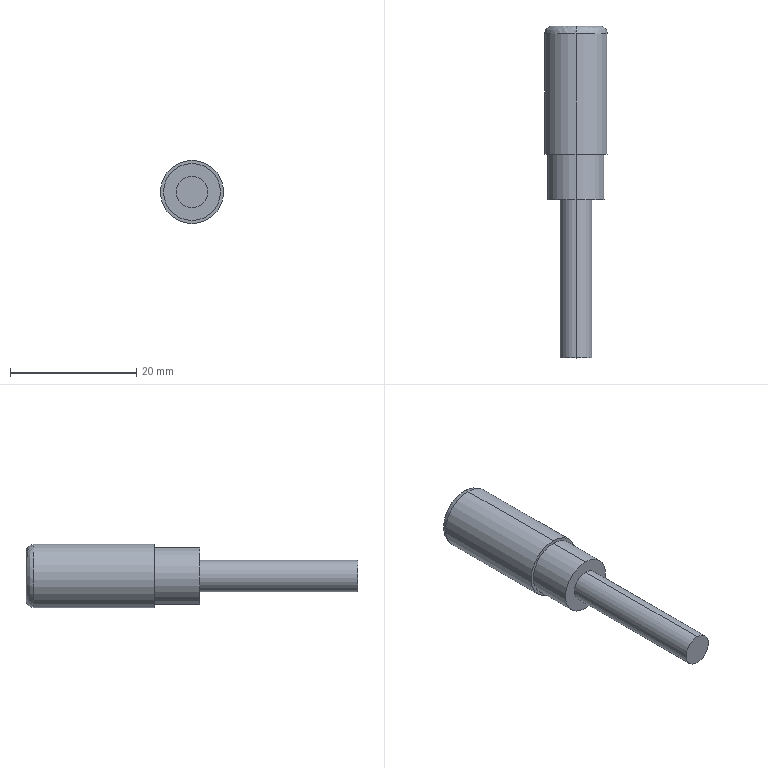Part | SolidWorks | features ICE 3, BaseBody 1 | 1 solid | 19 faces | box 10 x 52.5 x 10 mm | volume 2526 mm3 | plane 11 | cylinder 6 | spline 2 | commonest cylinder face diameters 5 x2 9 x2 10 x2
STEP:
#1=CARTESIAN_POINT('',(0.,24.5,3.8));
#2=VERTEX_POINT('',#1);
#3=CARTESIAN_POINT('',(0.,24.5,-3.8));
#4=VERTEX_POINT('',#3);
#5=CARTESIAN_POINT('',(0.,24.5,3.8));
#6=CARTESIAN_POINT('',(-7.6,24.5,3.8));
#7=CARTESIAN_POINT('',(-7.6,24.5,-3.8));
#8=CARTESIAN_POINT('',(0.,24.5,-3.8));
#9=(BOUNDED_CURVE()B_SPLINE_CURVE(3,(#5,#6,#7,#8),.UNSPECIFIED.,.F.,.F.)B_SPLINE_CURVE_WITH_KNOTS((4,4),(0.,1.),.UNSPECIFIED.)CURVE()GEOMETRIC_REPRESENTATION_ITEM()RATIONAL_B_SPLINE_CURVE((1.,0.3333,0.3333,1.))REPRESENTATION_ITEM(''));
#10=EDGE_CURVE('',#2,#4,#9,.T.);
#11=ORIENTED_EDGE('',*,*,#10,.T.);
#12=CARTESIAN_POINT('',(0.,23.3,-5.));
#13=VERTEX_POINT('',#12);
#14=CARTESIAN_POINT('',(0.,23.3,-3.8));
#15=DIRECTION('',(-1.,0.,0.));
#16=DIRECTION('',(0.,0.,-1.));
#17=AXIS2_PLACEMENT_3D('',#14,#15,#16);
#18=CIRCLE('',#17,1.2);
#19=EDGE_CURVE('',#4,#13,#18,.T.);
#20=ORIENTED_EDGE('',*,*,#19,.T.);
#21=CARTESIAN_POINT('',(0.,23.3,5.));
#22=VERTEX_POINT('',#21);
#23=CARTESIAN_POINT('',(0.,23.3,0.));
#24=DIRECTION('',(0.,-1.,0.));
#25=DIRECTION('',(0.,0.,-1.));
#26=AXIS2_PLACEMENT_3D('',#23,#24,#25);
#27=CIRCLE('',#26,5.);
#28=EDGE_CURVE('',#22,#13,#27,.T.);
#29=ORIENTED_EDGE('',*,*,#28,.F.);
#30=CARTESIAN_POINT('',(0.,23.3,3.8));
#31=DIRECTION('',(1.,0.,0.));
#32=DIRECTION('',(0.,0.,1.));
#33=AXIS2_PLACEMENT_3D('',#30,#31,#32);
#34=CIRCLE('',#33,1.2);
#35=EDGE_CURVE('',#2,#22,#34,.T.);
#36=ORIENTED_EDGE('',*,*,#35,.F.);
#37=EDGE_LOOP('',(#11,#20,#29,#36));
#38=FACE_OUTER_BOUND('',#37,.T.);
#39=CARTESIAN_POINT('',(0.,24.5,-3.8));
#40=CARTESIAN_POINT('',(-7.6,24.5,-3.8));
#41=CARTESIAN_POINT('',(-7.6,24.5,3.8));
#42=CARTESIAN_POINT('',(0.,24.5,3.8));
#43=CARTESIAN_POINT('',(0.,24.5,-4.503));
#44=CARTESIAN_POINT('',(-9.006,24.5,-4.503));
#45=CARTESIAN_POINT('',(-9.006,24.5,4.503));
#46=CARTESIAN_POINT('',(0.,24.5,4.503));
#47=CARTESIAN_POINT('',(0.,24.003,-5.));
#48=CARTESIAN_POINT('',(-10.,24.003,-5.));
#49=CARTESIAN_POINT('',(-10.,24.003,5.));
#50=CARTESIAN_POINT('',(0.,24.003,5.));
#51=CARTESIAN_POINT('',(0.,23.3,-5.));
#52=CARTESIAN_POINT('',(-10.,23.3,-5.));
#53=CARTESIAN_POINT('',(-10.,23.3,5.));
#54=CARTESIAN_POINT('',(0.,23.3,5.));
#55=(BOUNDED_SURFACE()B_SPLINE_SURFACE(3,3,((#39,#40,#41,#42),(#43,#44,#45,#46),(#47,#48,#49,#50),(#51,#52,#53,#54)),.UNSPECIFIED.,.F.,.F.,.F.)B_SPLINE_SURFACE_WITH_KNOTS((4,4),(4,4),(0.,1.),(0.,1.),.UNSPECIFIED.)GEOMETRIC_REPRESENTATION_ITEM()RATIONAL_B_SPLINE_SURFACE(((1.,0.3333,0.3333,1.),(0.8047,0.2682,0.2682,0.8047),(0.8047,0.2682,0.2682,0.8047),(1.,0.3333,0.3333,1.)))REPRESENTATION_ITEM('')SURFACE());
#56=ADVANCED_FACE('',(#38),#55,.T.);
#57=CARTESIAN_POINT('',(0.,-3.,2.5));
#58=VERTEX_POINT('',#57);
#59=CARTESIAN_POINT('',(0.,-3.,-2.5));
#60=VERTEX_POINT('',#59);
#61=CARTESIAN_POINT('',(0.,-3.,0.));
#62=DIRECTION('',(0.,1.,0.));
#63=DIRECTION('',(0.,0.,-1.));
#64=AXIS2_PLACEMENT_3D('',#61,#62,#63);
#65=CIRCLE('',#64,2.5);
#66=EDGE_CURVE('',#58,#60,#65,.T.);
#67=ORIENTED_EDGE('',*,*,#66,.F.);
#68=CARTESIAN_POINT('',(0.,-28.,2.5));
#69=VERTEX_POINT('',#68);
#70=CARTESIAN_POINT('',(0.,-12.284,2.5));
#71=DIRECTION('',(0.,-1.,0.));
#72=VECTOR('',#71,1000.);
#73=LINE('',#70,#72);
#74=EDGE_CURVE('',#58,#69,#73,.T.);
#75=ORIENTED_EDGE('',*,*,#74,.T.);
#76=CARTESIAN_POINT('',(0.,-28.,-2.5));
#77=VERTEX_POINT('',#76);
#78=CARTESIAN_POINT('',(0.,-28.,0.));
#79=DIRECTION('',(0.,-1.,0.));
#80=DIRECTION('',(0.,0.,-1.));
#81=AXIS2_PLACEMENT_3D('',#78,#79,#80);
#82=CIRCLE('',#81,2.5);
#83=EDGE_CURVE('',#77,#69,#82,.T.);
#84=ORIENTED_EDGE('',*,*,#83,.F.);
#85=CARTESIAN_POINT('',(0.,-12.284,-2.5));
#86=DIRECTION('',(0.,-1.,0.));
#87=VECTOR('',#86,1000.);
#88=LINE('',#85,#87);
#89=EDGE_CURVE('',#60,#77,#88,.T.);
#90=ORIENTED_EDGE('',*,*,#89,.F.);
#91=EDGE_LOOP('',(#67,#75,#84,#90));
#92=FACE_OUTER_BOUND('',#91,.T.);
#93=CARTESIAN_POINT('',(0.,-12.284,0.));
#94=DIRECTION('',(0.,-1.,0.));
#95=DIRECTION('',(0.,0.,-1.));
#96=AXIS2_PLACEMENT_3D('',#93,#94,#95);
#97=CYLINDRICAL_SURFACE('',#96,2.5);
#98=ADVANCED_FACE('',(#92),#97,.T.);
#99=CARTESIAN_POINT('',(0.,4.2,-4.5));
#100=VERTEX_POINT('',#99);
#101=CARTESIAN_POINT('',(0.,4.2,4.5));
#102=VERTEX_POINT('',#101);
#103=CARTESIAN_POINT('',(0.,4.2,0.));
#104=DIRECTION('',(0.,-1.,0.));
#105=DIRECTION('',(0.,0.,-1.));
#106=AXIS2_PLACEMENT_3D('',#103,#104,#105);
#107=CIRCLE('',#106,4.5);
#108=EDGE_CURVE('',#100,#102,#107,.T.);
#109=ORIENTED_EDGE('',*,*,#108,.T.);
#110=CARTESIAN_POINT('',(0.,-3.,4.5));
#111=VERTEX_POINT('',#110);
#112=CARTESIAN_POINT('',(0.,4.2,4.5));
#113=DIRECTION('',(0.,-1.,0.));
#114=VECTOR('',#113,1000.);
#115=LINE('',#112,#114);
#116=EDGE_CURVE('',#102,#111,#115,.T.);
#117=ORIENTED_EDGE('',*,*,#116,.T.);
#118=CARTESIAN_POINT('',(0.,-3.,-4.5));
#119=VERTEX_POINT('',#118);
#120=CARTESIAN_POINT('',(0.,-3.,0.));
#121=DIRECTION('',(0.,-1.,0.));
#122=DIRECTION('',(0.,0.,-1.));
#123=AXIS2_PLACEMENT_3D('',#120,#121,#122);
#124=CIRCLE('',#123,4.5);
#125=EDGE_CURVE('',#119,#111,#124,.T.);
#126=ORIENTED_EDGE('',*,*,#125,.F.);
#127=CARTESIAN_POINT('',(0.,4.2,-4.5));
#128=DIRECTION('',(0.,-1.,0.));
#129=VECTOR('',#128,1000.);
#130=LINE('',#127,#129);
#131=EDGE_CURVE('',#100,#119,#130,.T.);
#132=ORIENTED_EDGE('',*,*,#131,.F.);
#133=EDGE_LOOP('',(#109,#117,#126,#132));
#134=FACE_OUTER_BOUND('',#133,.T.);
#135=CARTESIAN_POINT('',(0.,4.2,0.));
#136=DIRECTION('',(0.,-1.,0.));
#137=DIRECTION('',(0.,0.,-1.));
#138=AXIS2_PLACEMENT_3D('',#135,#136,#137);
#139=CYLINDRICAL_SURFACE('',#138,4.5);
#140=ADVANCED_FACE('',(#134),#139,.T.);
#141=CARTESIAN_POINT('',(0.,23.3,0.));
#142=DIRECTION('',(0.,-1.,0.));
#143=DIRECTION('',(0.,0.,-1.));
#144=AXIS2_PLACEMENT_3D('',#141,#142,#143);
#145=CIRCLE('',#144,5.);
#146=EDGE_CURVE('',#13,#22,#145,.T.);
#147=ORIENTED_EDGE('',*,*,#146,.T.);
#148=CARTESIAN_POINT('',(0.,4.2,5.));
#149=VERTEX_POINT('',#148);
#150=CARTESIAN_POINT('',(0.,11.827,5.));
#151=DIRECTION('',(0.,-1.,0.));
#152=VECTOR('',#151,1000.);
#153=LINE('',#150,#152);
#154=EDGE_CURVE('',#22,#149,#153,.T.);
#155=ORIENTED_EDGE('',*,*,#154,.T.);
#156=CARTESIAN_POINT('',(0.,4.2,-5.));
#157=VERTEX_POINT('',#156);
#158=CARTESIAN_POINT('',(0.,4.2,0.));
#159=DIRECTION('',(0.,-1.,0.));
#160=DIRECTION('',(0.,0.,-1.));
#161=AXIS2_PLACEMENT_3D('',#158,#159,#160);
#162=CIRCLE('',#161,5.);
#163=EDGE_CURVE('',#157,#149,#162,.T.);
#164=ORIENTED_EDGE('',*,*,#163,.F.);
#165=CARTESIAN_POINT('',(0.,11.827,-5.));
#166=DIRECTION('',(0.,-1.,0.));
#167=VECTOR('',#166,1000.);
#168=LINE('',#165,#167);
#169=EDGE_CURVE('',#13,#157,#168,.T.);
#170=ORIENTED_EDGE('',*,*,#169,.F.);
#171=EDGE_LOOP('',(#147,#155,#164,#170));
#172=FACE_OUTER_BOUND('',#171,.T.);
#173=CARTESIAN_POINT('',(0.,11.827,0.));
#174=DIRECTION('',(0.,-1.,0.));
#175=DIRECTION('',(0.,0.,-1.));
#176=AXIS2_PLACEMENT_3D('',#173,#174,#175);
#177=CYLINDRICAL_SURFACE('',#176,5.);
#178=ADVANCED_FACE('',(#172),#177,.T.);
#179=ORIENTED_EDGE('',*,*,#154,.F.);
#180=ORIENTED_EDGE('',*,*,#28,.T.);
#181=ORIENTED_EDGE('',*,*,#169,.T.);
#182=CARTESIAN_POINT('',(0.,4.2,0.));
#183=DIRECTION('',(0.,-1.,0.));
#184=DIRECTION('',(0.,0.,-1.));
#185=AXIS2_PLACEMENT_3D('',#182,#183,#184);
#186=CIRCLE('',#185,5.);
#187=EDGE_CURVE('',#149,#157,#186,.T.);
#188=ORIENTED_EDGE('',*,*,#187,.F.);
#189=EDGE_LOOP('',(#179,#180,#181,#188));
#190=FACE_OUTER_BOUND('',#189,.T.);
#191=CARTESIAN_POINT('',(0.,11.827,0.));
#192=DIRECTION('',(0.,-1.,0.));
#193=DIRECTION('',(0.,0.,-1.));
#194=AXIS2_PLACEMENT_3D('',#191,#192,#193);
#195=CYLINDRICAL_SURFACE('',#194,5.);
#196=ADVANCED_FACE('',(#190),#195,.T.);
#197=ORIENTED_EDGE('',*,*,#19,.F.);
#198=CARTESIAN_POINT('',(3.8,24.5,0.));
#199=VERTEX_POINT('',#198);
#200=CARTESIAN_POINT('',(0.,24.5,-3.8));
#201=CARTESIAN_POINT('',(2.226,24.5,-3.8));
#202=CARTESIAN_POINT('',(3.8,24.5,-2.226));
#203=CARTESIAN_POINT('',(3.8,24.5,0.));
#204=(BOUNDED_CURVE()B_SPLINE_CURVE(3,(#200,#201,#202,#203),.UNSPECIFIED.,.F.,.F.)B_SPLINE_CURVE_WITH_KNOTS((4,4),(0.,1.),.UNSPECIFIED.)CURVE()GEOMETRIC_REPRESENTATION_ITEM()RATIONAL_B_SPLINE_CURVE((1.,0.8047,0.8047,1.))REPRESENTATION_ITEM(''));
#205=EDGE_CURVE('',#4,#199,#204,.T.);
#206=ORIENTED_EDGE('',*,*,#205,.T.);
#207=CARTESIAN_POINT('',(3.8,24.5,0.));
#208=CARTESIAN_POINT('',(3.8,24.5,2.226));
#209=CARTESIAN_POINT('',(2.226,24.5,3.8));
#210=CARTESIAN_POINT('',(0.,24.5,3.8));
#211=(BOUNDED_CURVE()B_SPLINE_CURVE(3,(#207,#208,#209,#210),.UNSPECIFIED.,.F.,.F.)B_SPLINE_CURVE_WITH_KNOTS((4,4),(0.,1.),.UNSPECIFIED.)CURVE()GEOMETRIC_REPRESENTATION_ITEM()RATIONAL_B_SPLINE_CURVE((1.,0.8047,0.8047,1.))REPRESENTATION_ITEM(''));
#212=EDGE_CURVE('',#199,#2,#211,.T.);
#213=ORIENTED_EDGE('',*,*,#212,.T.);
#214=ORIENTED_EDGE('',*,*,#35,.T.);
#215=ORIENTED_EDGE('',*,*,#146,.F.);
#216=EDGE_LOOP('',(#197,#206,#213,#214,#215));
#217=FACE_OUTER_BOUND('',#216,.T.);
#218=CARTESIAN_POINT('',(0.,24.5,3.8));
#219=CARTESIAN_POINT('',(7.6,24.5,3.8));
#220=CARTESIAN_POINT('',(7.6,24.5,-3.8));
#221=CARTESIAN_POINT('',(0.,24.5,-3.8));
#222=CARTESIAN_POINT('',(0.,24.5,4.503));
#223=CARTESIAN_POINT('',(9.006,24.5,4.503));
#224=CARTESIAN_POINT('',(9.006,24.5,-4.503));
#225=CARTESIAN_POINT('',(0.,24.5,-4.503));
#226=CARTESIAN_POINT('',(0.,24.003,5.));
#227=CARTESIAN_POINT('',(10.,24.003,5.));
#228=CARTESIAN_POINT('',(10.,24.003,-5.));
#229=CARTESIAN_POINT('',(0.,24.003,-5.));
#230=CARTESIAN_POINT('',(0.,23.3,5.));
#231=CARTESIAN_POINT('',(10.,23.3,5.));
#232=CARTESIAN_POINT('',(10.,23.3,-5.));
#233=CARTESIAN_POINT('',(0.,23.3,-5.));
#234=(BOUNDED_SURFACE()B_SPLINE_SURFACE(3,3,((#218,#219,#220,#221),(#222,#223,#224,#225),(#226,#227,#228,#229),(#230,#231,#232,#233)),.UNSPECIFIED.,.F.,.F.,.F.)B_SPLINE_SURFACE_WITH_KNOTS((4,4),(4,4),(0.,1.),(0.,1.),.UNSPECIFIED.)GEOMETRIC_REPRESENTATION_ITEM()RATIONAL_B_SPLINE_SURFACE(((1.,0.3333,0.3333,1.),(0.8047,0.2682,0.2682,0.8047),(0.8047,0.2682,0.2682,0.8047),(1.,0.3333,0.3333,1.)))REPRESENTATION_ITEM('')SURFACE());
#235=ADVANCED_FACE('',(#217),#234,.T.);
#236=ORIENTED_EDGE('',*,*,#10,.F.);
#237=ORIENTED_EDGE('',*,*,#212,.F.);
#238=ORIENTED_EDGE('',*,*,#205,.F.);
#239=EDGE_LOOP('',(#236,#237,#238));
#240=FACE_OUTER_BOUND('',#239,.T.);
#241=CARTESIAN_POINT('',(1.5,24.5,-0.866));
#242=VERTEX_POINT('',#241);
#243=CARTESIAN_POINT('',(1.5,24.5,0.866));
#244=VERTEX_POINT('',#243);
#245=CARTESIAN_POINT('',(1.5,24.5,0.));
#246=DIRECTION('',(0.,0.,1.));
#247=VECTOR('',#246,1000.);
#248=LINE('',#245,#247);
#249=EDGE_CURVE('',#242,#244,#248,.T.);
#250=ORIENTED_EDGE('',*,*,#249,.T.);
#251=CARTESIAN_POINT('',(0.,24.5,1.732));
#252=VERTEX_POINT('',#251);
#253=CARTESIAN_POINT('',(1.5,24.5,0.866));
#254=DIRECTION('',(-0.866,0.,0.5));
#255=VECTOR('',#254,1000.);
#256=LINE('',#253,#255);
#257=EDGE_CURVE('',#244,#252,#256,.T.);
#258=ORIENTED_EDGE('',*,*,#257,.T.);
#259=CARTESIAN_POINT('',(-1.5,24.5,0.866));
#260=VERTEX_POINT('',#259);
#261=CARTESIAN_POINT('',(0.,24.5,1.732));
#262=DIRECTION('',(-0.866,0.,-0.5));
#263=VECTOR('',#262,1000.);
#264=LINE('',#261,#263);
#265=EDGE_CURVE('',#252,#260,#264,.T.);
#266=ORIENTED_EDGE('',*,*,#265,.T.);
#267=CARTESIAN_POINT('',(-1.5,24.5,-0.866));
#268=VERTEX_POINT('',#267);
#269=CARTESIAN_POINT('',(-1.5,24.5,0.));
#270=DIRECTION('',(0.,0.,-1.));
#271=VECTOR('',#270,1000.);
#272=LINE('',#269,#271);
#273=EDGE_CURVE('',#260,#268,#272,.T.);
#274=ORIENTED_EDGE('',*,*,#273,.T.);
#275=CARTESIAN_POINT('',(0.,24.5,-1.732));
#276=VERTEX_POINT('',#275);
#277=CARTESIAN_POINT('',(-1.5,24.5,-0.866));
#278=DIRECTION('',(0.866,0.,-0.5));
#279=VECTOR('',#278,1000.);
#280=LINE('',#277,#279);
#281=EDGE_CURVE('',#268,#276,#280,.T.);
#282=ORIENTED_EDGE('',*,*,#281,.T.);
#283=CARTESIAN_POINT('',(0.,24.5,-1.732));
#284=DIRECTION('',(0.866,0.,0.5));
#285=VECTOR('',#284,1000.);
#286=LINE('',#283,#285);
#287=EDGE_CURVE('',#276,#242,#286,.T.);
#288=ORIENTED_EDGE('',*,*,#287,.T.);
#289=EDGE_LOOP('',(#250,#258,#266,#274,#282,#288));
#290=FACE_BOUND('',#289,.T.);
#291=CARTESIAN_POINT('',(1.9,24.5,0.));
#292=DIRECTION('',(0.,1.,0.));
#293=DIRECTION('',(0.,0.,1.));
#294=AXIS2_PLACEMENT_3D('',#291,#292,#293);
#295=PLANE('',#294);
#296=ADVANCED_FACE('',(#240,#290),#295,.T.);
#297=CARTESIAN_POINT('',(0.,23.45,1.732));
#298=VERTEX_POINT('',#297);
#299=CARTESIAN_POINT('',(0.,24.5,1.732));
#300=DIRECTION('',(0.,-1.,0.));
#301=VECTOR('',#300,1000.);
#302=LINE('',#299,#301);
#303=EDGE_CURVE('',#252,#298,#302,.T.);
#304=ORIENTED_EDGE('',*,*,#303,.F.);
#305=ORIENTED_EDGE('',*,*,#257,.F.);
#306=CARTESIAN_POINT('',(1.5,23.45,0.866));
#307=VERTEX_POINT('',#306);
#308=CARTESIAN_POINT('',(1.5,24.5,0.866));
#309=DIRECTION('',(0.,1.,0.));
#310=VECTOR('',#309,1000.);
#311=LINE('',#308,#310);
#312=EDGE_CURVE('',#307,#244,#311,.T.);
#313=ORIENTED_EDGE('',*,*,#312,.F.);
#314=CARTESIAN_POINT('',(0.,23.45,1.732));
#315=DIRECTION('',(0.866,0.,-0.5));
#316=VECTOR('',#315,1000.);
#317=LINE('',#314,#316);
#318=EDGE_CURVE('',#298,#307,#317,.T.);
#319=ORIENTED_EDGE('',*,*,#318,.F.);
#320=EDGE_LOOP('',(#304,#305,#313,#319));
#321=FACE_OUTER_BOUND('',#320,.T.);
#322=CARTESIAN_POINT('',(0.,24.5,1.732));
#323=DIRECTION('',(0.5,0.,0.866));
#324=DIRECTION('',(0.866,0.,-0.5));
#325=AXIS2_PLACEMENT_3D('',#322,#323,#324);
#326=PLANE('',#325);
#327=ADVANCED_FACE('',(#321),#326,.F.);
#328=ORIENTED_EDGE('',*,*,#312,.T.);
#329=ORIENTED_EDGE('',*,*,#249,.F.);
#330=CARTESIAN_POINT('',(1.5,23.45,-0.866));
#331=VERTEX_POINT('',#330);
#332=CARTESIAN_POINT('',(1.5,24.5,-0.866));
#333=DIRECTION('',(0.,1.,0.));
#334=VECTOR('',#333,1000.);
#335=LINE('',#332,#334);
#336=EDGE_CURVE('',#331,#242,#335,.T.);
#337=ORIENTED_EDGE('',*,*,#336,.F.);
#338=CARTESIAN_POINT('',(1.5,23.45,0.866));
#339=DIRECTION('',(0.,0.,-1.));
#340=VECTOR('',#339,1000.);
#341=LINE('',#338,#340);
#342=EDGE_CURVE('',#307,#331,#341,.T.);
#343=ORIENTED_EDGE('',*,*,#342,.F.);
#344=EDGE_LOOP('',(#328,#329,#337,#343));
#345=FACE_OUTER_BOUND('',#344,.T.);
#346=CARTESIAN_POINT('',(1.5,24.5,0.866));
#347=DIRECTION('',(1.,0.,0.));
#348=DIRECTION('',(0.,0.,-1.));
#349=AXIS2_PLACEMENT_3D('',#346,#347,#348);
#350=PLANE('',#349);
#351=ADVANCED_FACE('',(#345),#350,.F.);
#352=ORIENTED_EDGE('',*,*,#336,.T.);
#353=ORIENTED_EDGE('',*,*,#287,.F.);
#354=CARTESIAN_POINT('',(0.,23.45,-1.732));
#355=VERTEX_POINT('',#354);
#356=CARTESIAN_POINT('',(0.,24.5,-1.732));
#357=DIRECTION('',(0.,1.,0.));
#358=VECTOR('',#357,1000.);
#359=LINE('',#356,#358);
#360=EDGE_CURVE('',#355,#276,#359,.T.);
#361=ORIENTED_EDGE('',*,*,#360,.F.);
#362=CARTESIAN_POINT('',(1.5,23.45,-0.866));
#363=DIRECTION('',(-0.866,0.,-0.5));
#364=VECTOR('',#363,1000.);
#365=LINE('',#362,#364);
#366=EDGE_CURVE('',#331,#355,#365,.T.);
#367=ORIENTED_EDGE('',*,*,#366,.F.);
#368=EDGE_LOOP('',(#352,#353,#361,#367));
#369=FACE_OUTER_BOUND('',#368,.T.);
#370=CARTESIAN_POINT('',(1.5,24.5,-0.866));
#371=DIRECTION('',(0.5,0.,-0.866));
#372=DIRECTION('',(-0.866,0.,-0.5));
#373=AXIS2_PLACEMENT_3D('',#370,#371,#372);
#374=PLANE('',#373);
#375=ADVANCED_FACE('',(#369),#374,.F.);
#376=ORIENTED_EDGE('',*,*,#360,.T.);
#377=ORIENTED_EDGE('',*,*,#281,.F.);
#378=CARTESIAN_POINT('',(-1.5,23.45,-0.866));
#379=VERTEX_POINT('',#378);
#380=CARTESIAN_POINT('',(-1.5,24.5,-0.866));
#381=DIRECTION('',(0.,1.,0.));
#382=VECTOR('',#381,1000.);
#383=LINE('',#380,#382);
#384=EDGE_CURVE('',#379,#268,#383,.T.);
#385=ORIENTED_EDGE('',*,*,#384,.F.);
#386=CARTESIAN_POINT('',(0.,23.45,-1.732));
#387=DIRECTION('',(-0.866,0.,0.5));
#388=VECTOR('',#387,1000.);
#389=LINE('',#386,#388);
#390=EDGE_CURVE('',#355,#379,#389,.T.);
#391=ORIENTED_EDGE('',*,*,#390,.F.);
#392=EDGE_LOOP('',(#376,#377,#385,#391));
#393=FACE_OUTER_BOUND('',#392,.T.);
#394=CARTESIAN_POINT('',(0.,24.5,-1.732));
#395=DIRECTION('',(-0.5,0.,-0.866));
#396=DIRECTION('',(-0.866,0.,0.5));
#397=AXIS2_PLACEMENT_3D('',#394,#395,#396);
#398=PLANE('',#397);
#399=ADVANCED_FACE('',(#393),#398,.F.);
#400=ORIENTED_EDGE('',*,*,#384,.T.);
#401=ORIENTED_EDGE('',*,*,#273,.F.);
#402=CARTESIAN_POINT('',(-1.5,23.45,0.866));
#403=VERTEX_POINT('',#402);
#404=CARTESIAN_POINT('',(-1.5,24.5,0.866));
#405=DIRECTION('',(0.,1.,0.));
#406=VECTOR('',#405,1000.);
#407=LINE('',#404,#406);
#408=EDGE_CURVE('',#403,#260,#407,.T.);
#409=ORIENTED_EDGE('',*,*,#408,.F.);
#410=CARTESIAN_POINT('',(-1.5,23.45,-0.866));
#411=DIRECTION('',(0.,0.,1.));
#412=VECTOR('',#411,1000.);
#413=LINE('',#410,#412);
#414=EDGE_CURVE('',#379,#403,#413,.T.);
#415=ORIENTED_EDGE('',*,*,#414,.F.);
#416=EDGE_LOOP('',(#400,#401,#409,#415));
#417=FACE_OUTER_BOUND('',#416,.T.);
#418=CARTESIAN_POINT('',(-1.5,24.5,-0.866));
#419=DIRECTION('',(-1.,0.,0.));
#420=DIRECTION('',(0.,0.,1.));
#421=AXIS2_PLACEMENT_3D('',#418,#419,#420);
#422=PLANE('',#421);
#423=ADVANCED_FACE('',(#417),#422,.F.);
#424=ORIENTED_EDGE('',*,*,#408,.T.);
#425=ORIENTED_EDGE('',*,*,#265,.F.);
#426=ORIENTED_EDGE('',*,*,#303,.T.);
#427=CARTESIAN_POINT('',(-1.5,23.45,0.866));
#428=DIRECTION('',(0.866,0.,0.5));
#429=VECTOR('',#428,1000.);
#430=LINE('',#427,#429);
#431=EDGE_CURVE('',#403,#298,#430,.T.);
#432=ORIENTED_EDGE('',*,*,#431,.F.);
#433=EDGE_LOOP('',(#424,#425,#426,#432));
#434=FACE_OUTER_BOUND('',#433,.T.);
#435=CARTESIAN_POINT('',(-1.5,24.5,0.866));
#436=DIRECTION('',(-0.5,0.,0.866));
#437=DIRECTION('',(0.866,0.,0.5));
#438=AXIS2_PLACEMENT_3D('',#435,#436,#437);
#439=PLANE('',#438);
#440=ADVANCED_FACE('',(#434),#439,.F.);
#441=ORIENTED_EDGE('',*,*,#390,.T.);
#442=ORIENTED_EDGE('',*,*,#414,.T.);
#443=ORIENTED_EDGE('',*,*,#431,.T.);
#444=ORIENTED_EDGE('',*,*,#318,.T.);
#445=ORIENTED_EDGE('',*,*,#342,.T.);
#446=ORIENTED_EDGE('',*,*,#366,.T.);
#447=EDGE_LOOP('',(#441,#442,#443,#444,#445,#446));
#448=FACE_OUTER_BOUND('',#447,.T.);
#449=CARTESIAN_POINT('',(0.,23.45,0.));
#450=DIRECTION('',(0.,1.,0.));
#451=DIRECTION('',(0.,0.,1.));
#452=AXIS2_PLACEMENT_3D('',#449,#450,#451);
#453=PLANE('',#452);
#454=ADVANCED_FACE('',(#448),#453,.T.);
#455=ORIENTED_EDGE('',*,*,#108,.F.);
#456=CARTESIAN_POINT('',(0.,4.2,0.));
#457=DIRECTION('',(0.,-1.,0.));
#458=DIRECTION('',(0.,0.,-1.));
#459=AXIS2_PLACEMENT_3D('',#456,#457,#458);
#460=CIRCLE('',#459,4.5);
#461=EDGE_CURVE('',#102,#100,#460,.T.);
#462=ORIENTED_EDGE('',*,*,#461,.F.);
#463=EDGE_LOOP('',(#455,#462));
#464=FACE_BOUND('',#463,.T.);
#465=ORIENTED_EDGE('',*,*,#163,.T.);
#466=ORIENTED_EDGE('',*,*,#187,.T.);
#467=EDGE_LOOP('',(#465,#466));
#468=FACE_OUTER_BOUND('',#467,.T.);
#469=CARTESIAN_POINT('',(0.,4.2,0.));
#470=DIRECTION('',(0.,-1.,0.));
#471=DIRECTION('',(0.,0.,-1.));
#472=AXIS2_PLACEMENT_3D('',#469,#470,#471);
#473=PLANE('',#472);
#474=ADVANCED_FACE('',(#464,#468),#473,.T.);
#475=ORIENTED_EDGE('',*,*,#116,.F.);
#476=ORIENTED_EDGE('',*,*,#461,.T.);
#477=ORIENTED_EDGE('',*,*,#131,.T.);
#478=CARTESIAN_POINT('',(0.,-3.,0.));
#479=DIRECTION('',(0.,-1.,0.));
#480=DIRECTION('',(0.,0.,-1.));
#481=AXIS2_PLACEMENT_3D('',#478,#479,#480);
#482=CIRCLE('',#481,4.5);
#483=EDGE_CURVE('',#111,#119,#482,.T.);
#484=ORIENTED_EDGE('',*,*,#483,.F.);
#485=EDGE_LOOP('',(#475,#476,#477,#484));
#486=FACE_OUTER_BOUND('',#485,.T.);
#487=CARTESIAN_POINT('',(0.,4.2,0.));
#488=DIRECTION('',(0.,-1.,0.));
#489=DIRECTION('',(0.,0.,-1.));
#490=AXIS2_PLACEMENT_3D('',#487,#488,#489);
#491=CYLINDRICAL_SURFACE('',#490,4.5);
#492=ADVANCED_FACE('',(#486),#491,.T.);
#493=ORIENTED_EDGE('',*,*,#83,.T.);
#494=CARTESIAN_POINT('',(0.,-28.,0.));
#495=DIRECTION('',(0.,-1.,0.));
#496=DIRECTION('',(0.,0.,-1.));
#497=AXIS2_PLACEMENT_3D('',#494,#495,#496);
#498=CIRCLE('',#497,2.5);
#499=EDGE_CURVE('',#69,#77,#498,.T.);
#500=ORIENTED_EDGE('',*,*,#499,.T.);
#501=EDGE_LOOP('',(#493,#500));
#502=FACE_OUTER_BOUND('',#501,.T.);
#503=CARTESIAN_POINT('',(0.,-28.,0.));
#504=DIRECTION('',(0.,-1.,0.));
#505=DIRECTION('',(0.,0.,-1.));
#506=AXIS2_PLACEMENT_3D('',#503,#504,#505);
#507=PLANE('',#506);
#508=ADVANCED_FACE('',(#502),#507,.T.);
#509=ORIENTED_EDGE('',*,*,#74,.F.);
#510=CARTESIAN_POINT('',(0.,-3.,0.));
#511=DIRECTION('',(0.,1.,0.));
#512=DIRECTION('',(0.,0.,-1.));
#513=AXIS2_PLACEMENT_3D('',#510,#511,#512);
#514=CIRCLE('',#513,2.5);
#515=EDGE_CURVE('',#60,#58,#514,.T.);
#516=ORIENTED_EDGE('',*,*,#515,.F.);
#517=ORIENTED_EDGE('',*,*,#89,.T.);
#518=ORIENTED_EDGE('',*,*,#499,.F.);
#519=EDGE_LOOP('',(#509,#516,#517,#518));
#520=FACE_OUTER_BOUND('',#519,.T.);
#521=CARTESIAN_POINT('',(0.,-12.284,0.));
#522=DIRECTION('',(0.,-1.,0.));
#523=DIRECTION('',(0.,0.,-1.));
#524=AXIS2_PLACEMENT_3D('',#521,#522,#523);
#525=CYLINDRICAL_SURFACE('',#524,2.5);
#526=ADVANCED_FACE('',(#520),#525,.T.);
#527=ORIENTED_EDGE('',*,*,#515,.T.);
#528=ORIENTED_EDGE('',*,*,#66,.T.);
#529=EDGE_LOOP('',(#527,#528));
#530=FACE_BOUND('',#529,.T.);
#531=ORIENTED_EDGE('',*,*,#125,.T.);
#532=ORIENTED_EDGE('',*,*,#483,.T.);
#533=EDGE_LOOP('',(#531,#532));
#534=FACE_OUTER_BOUND('',#533,.T.);
#535=CARTESIAN_POINT('',(0.,-3.,0.));
#536=DIRECTION('',(0.,-1.,0.));
#537=DIRECTION('',(0.,0.,-1.));
#538=AXIS2_PLACEMENT_3D('',#535,#536,#537);
#539=PLANE('',#538);
#540=ADVANCED_FACE('',(#530,#534),#539,.T.);
#541=CLOSED_SHELL('',(#56,#98,#140,#178,#196,#235,#296,#327,#351,#375,#399,#423,#440,#454,#474,#492,#508,#526,#540));
#542=MANIFOLD_SOLID_BREP('',#541);
#543=CARTESIAN_POINT('',(0.,0.,0.));
#544=DIRECTION('',(0.,0.,1.));
#545=DIRECTION('',(1.,0.,0.));
#546=AXIS2_PLACEMENT_3D('',#543,#544,#545);
#547=(LENGTH_UNIT()NAMED_UNIT(*)SI_UNIT(.MILLI.,.METRE.));
#548=UNCERTAINTY_MEASURE_WITH_UNIT(LENGTH_MEASURE(0.00001),#547,'','');
#549=(NAMED_UNIT(*)PLANE_ANGLE_UNIT()SI_UNIT($,.RADIAN.));
#550=(NAMED_UNIT(*)SI_UNIT($,.STERADIAN.)SOLID_ANGLE_UNIT());
#551=(GEOMETRIC_REPRESENTATION_CONTEXT(3)GLOBAL_UNCERTAINTY_ASSIGNED_CONTEXT((#548))GLOBAL_UNIT_ASSIGNED_CONTEXT((#547,#549,#550))REPRESENTATION_CONTEXT('',''));
#552=ADVANCED_BREP_SHAPE_REPRESENTATION('',(#542,#546),#551);